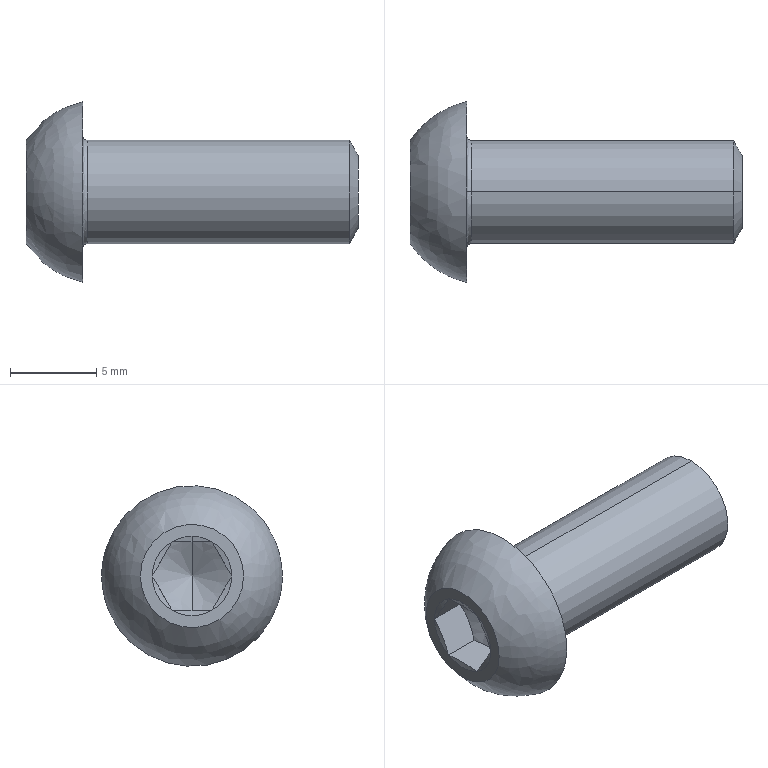Part | STEP file | 1 solid | 25 faces | box 19.3 x 10.5 x 10.5 mm | volume 623.745 mm3 | cone 11 | plane 9 | spline 3 | cylinder 2 | commonest cylinder face diameters 6 x2